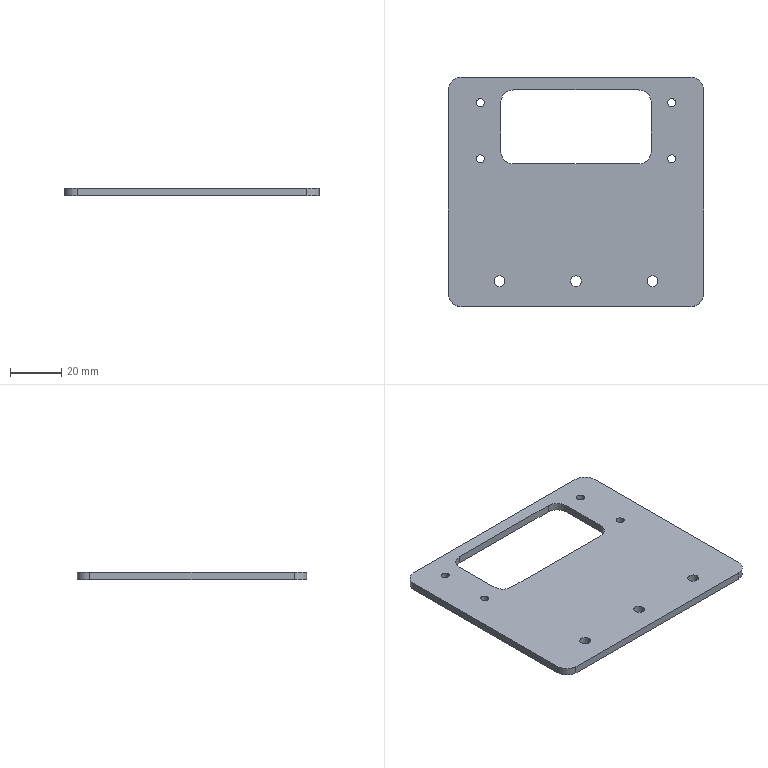Part | SolidWorks | features BaseBody 1 | 1 solid | 32 faces | box 100 x 90 x 3 mm | volume 21646 mm3 | cylinder 22 | plane 10 | commonest cylinder face diameters 3.2 x8 10 x8 4.2 x6
STEP:
#1=CARTESIAN_POINT('',(2.1,-35.,3.));
#2=VERTEX_POINT('',#1);
#3=CARTESIAN_POINT('',(-2.1,-35.,3.));
#4=VERTEX_POINT('',#3);
#5=CARTESIAN_POINT('',(0.,-35.,3.));
#6=DIRECTION('',(0.,0.,-1.));
#7=DIRECTION('',(-1.,0.,0.));
#8=AXIS2_PLACEMENT_3D('',#5,#6,#7);
#9=CIRCLE('',#8,2.1);
#10=EDGE_CURVE('',#2,#4,#9,.T.);
#11=ORIENTED_EDGE('',*,*,#10,.F.);
#12=CARTESIAN_POINT('',(2.1,-35.,0.));
#13=VERTEX_POINT('',#12);
#14=CARTESIAN_POINT('',(2.1,-35.,3.));
#15=DIRECTION('',(0.,0.,-1.));
#16=VECTOR('',#15,1000.);
#17=LINE('',#14,#16);
#18=EDGE_CURVE('',#2,#13,#17,.T.);
#19=ORIENTED_EDGE('',*,*,#18,.T.);
#20=CARTESIAN_POINT('',(-2.1,-35.,0.));
#21=VERTEX_POINT('',#20);
#22=CARTESIAN_POINT('',(0.,-35.,0.));
#23=DIRECTION('',(0.,0.,1.));
#24=DIRECTION('',(-1.,0.,0.));
#25=AXIS2_PLACEMENT_3D('',#22,#23,#24);
#26=CIRCLE('',#25,2.1);
#27=EDGE_CURVE('',#21,#13,#26,.T.);
#28=ORIENTED_EDGE('',*,*,#27,.F.);
#29=CARTESIAN_POINT('',(-2.1,-35.,3.));
#30=DIRECTION('',(0.,0.,-1.));
#31=VECTOR('',#30,1000.);
#32=LINE('',#29,#31);
#33=EDGE_CURVE('',#4,#21,#32,.T.);
#34=ORIENTED_EDGE('',*,*,#33,.F.);
#35=EDGE_LOOP('',(#11,#19,#28,#34));
#36=FACE_OUTER_BOUND('',#35,.T.);
#37=CARTESIAN_POINT('',(0.,-35.,3.));
#38=DIRECTION('',(0.,0.,-1.));
#39=DIRECTION('',(-1.,0.,0.));
#40=AXIS2_PLACEMENT_3D('',#37,#38,#39);
#41=CYLINDRICAL_SURFACE('',#40,2.1);
#42=ADVANCED_FACE('',(#36),#41,.F.);
#43=CARTESIAN_POINT('',(32.1,-35.,3.));
#44=VERTEX_POINT('',#43);
#45=CARTESIAN_POINT('',(27.9,-35.,3.));
#46=VERTEX_POINT('',#45);
#47=CARTESIAN_POINT('',(30.,-35.,3.));
#48=DIRECTION('',(0.,0.,-1.));
#49=DIRECTION('',(-1.,0.,0.));
#50=AXIS2_PLACEMENT_3D('',#47,#48,#49);
#51=CIRCLE('',#50,2.1);
#52=EDGE_CURVE('',#44,#46,#51,.T.);
#53=ORIENTED_EDGE('',*,*,#52,.F.);
#54=CARTESIAN_POINT('',(32.1,-35.,0.));
#55=VERTEX_POINT('',#54);
#56=CARTESIAN_POINT('',(32.1,-35.,3.));
#57=DIRECTION('',(0.,0.,-1.));
#58=VECTOR('',#57,1000.);
#59=LINE('',#56,#58);
#60=EDGE_CURVE('',#44,#55,#59,.T.);
#61=ORIENTED_EDGE('',*,*,#60,.T.);
#62=CARTESIAN_POINT('',(27.9,-35.,0.));
#63=VERTEX_POINT('',#62);
#64=CARTESIAN_POINT('',(30.,-35.,0.));
#65=DIRECTION('',(0.,0.,1.));
#66=DIRECTION('',(-1.,0.,0.));
#67=AXIS2_PLACEMENT_3D('',#64,#65,#66);
#68=CIRCLE('',#67,2.1);
#69=EDGE_CURVE('',#63,#55,#68,.T.);
#70=ORIENTED_EDGE('',*,*,#69,.F.);
#71=CARTESIAN_POINT('',(27.9,-35.,3.));
#72=DIRECTION('',(0.,0.,-1.));
#73=VECTOR('',#72,1000.);
#74=LINE('',#71,#73);
#75=EDGE_CURVE('',#46,#63,#74,.T.);
#76=ORIENTED_EDGE('',*,*,#75,.F.);
#77=EDGE_LOOP('',(#53,#61,#70,#76));
#78=FACE_OUTER_BOUND('',#77,.T.);
#79=CARTESIAN_POINT('',(30.,-35.,3.));
#80=DIRECTION('',(0.,0.,-1.));
#81=DIRECTION('',(-1.,0.,0.));
#82=AXIS2_PLACEMENT_3D('',#79,#80,#81);
#83=CYLINDRICAL_SURFACE('',#82,2.1);
#84=ADVANCED_FACE('',(#78),#83,.F.);
#85=CARTESIAN_POINT('',(39.1,13.,3.));
#86=VERTEX_POINT('',#85);
#87=CARTESIAN_POINT('',(35.9,13.,3.));
#88=VERTEX_POINT('',#87);
#89=CARTESIAN_POINT('',(37.5,13.,3.));
#90=DIRECTION('',(0.,0.,-1.));
#91=DIRECTION('',(-1.,0.,0.));
#92=AXIS2_PLACEMENT_3D('',#89,#90,#91);
#93=CIRCLE('',#92,1.6);
#94=EDGE_CURVE('',#86,#88,#93,.T.);
#95=ORIENTED_EDGE('',*,*,#94,.F.);
#96=CARTESIAN_POINT('',(39.1,13.,0.));
#97=VERTEX_POINT('',#96);
#98=CARTESIAN_POINT('',(39.1,13.,3.));
#99=DIRECTION('',(0.,0.,-1.));
#100=VECTOR('',#99,1000.);
#101=LINE('',#98,#100);
#102=EDGE_CURVE('',#86,#97,#101,.T.);
#103=ORIENTED_EDGE('',*,*,#102,.T.);
#104=CARTESIAN_POINT('',(35.9,13.,0.));
#105=VERTEX_POINT('',#104);
#106=CARTESIAN_POINT('',(37.5,13.,0.));
#107=DIRECTION('',(0.,0.,1.));
#108=DIRECTION('',(-1.,0.,0.));
#109=AXIS2_PLACEMENT_3D('',#106,#107,#108);
#110=CIRCLE('',#109,1.6);
#111=EDGE_CURVE('',#105,#97,#110,.T.);
#112=ORIENTED_EDGE('',*,*,#111,.F.);
#113=CARTESIAN_POINT('',(35.9,13.,3.));
#114=DIRECTION('',(0.,0.,-1.));
#115=VECTOR('',#114,1000.);
#116=LINE('',#113,#115);
#117=EDGE_CURVE('',#88,#105,#116,.T.);
#118=ORIENTED_EDGE('',*,*,#117,.F.);
#119=EDGE_LOOP('',(#95,#103,#112,#118));
#120=FACE_OUTER_BOUND('',#119,.T.);
#121=CARTESIAN_POINT('',(37.5,13.,3.));
#122=DIRECTION('',(0.,0.,-1.));
#123=DIRECTION('',(-1.,0.,0.));
#124=AXIS2_PLACEMENT_3D('',#121,#122,#123);
#125=CYLINDRICAL_SURFACE('',#124,1.6);
#126=ADVANCED_FACE('',(#120),#125,.F.);
#127=CARTESIAN_POINT('',(-35.9,13.,3.));
#128=VERTEX_POINT('',#127);
#129=CARTESIAN_POINT('',(-39.1,13.,3.));
#130=VERTEX_POINT('',#129);
#131=CARTESIAN_POINT('',(-37.5,13.,3.));
#132=DIRECTION('',(0.,0.,-1.));
#133=DIRECTION('',(-1.,0.,0.));
#134=AXIS2_PLACEMENT_3D('',#131,#132,#133);
#135=CIRCLE('',#134,1.6);
#136=EDGE_CURVE('',#128,#130,#135,.T.);
#137=ORIENTED_EDGE('',*,*,#136,.F.);
#138=CARTESIAN_POINT('',(-35.9,13.,0.));
#139=VERTEX_POINT('',#138);
#140=CARTESIAN_POINT('',(-35.9,13.,3.));
#141=DIRECTION('',(0.,0.,-1.));
#142=VECTOR('',#141,1000.);
#143=LINE('',#140,#142);
#144=EDGE_CURVE('',#128,#139,#143,.T.);
#145=ORIENTED_EDGE('',*,*,#144,.T.);
#146=CARTESIAN_POINT('',(-39.1,13.,0.));
#147=VERTEX_POINT('',#146);
#148=CARTESIAN_POINT('',(-37.5,13.,0.));
#149=DIRECTION('',(0.,0.,1.));
#150=DIRECTION('',(-1.,0.,0.));
#151=AXIS2_PLACEMENT_3D('',#148,#149,#150);
#152=CIRCLE('',#151,1.6);
#153=EDGE_CURVE('',#147,#139,#152,.T.);
#154=ORIENTED_EDGE('',*,*,#153,.F.);
#155=CARTESIAN_POINT('',(-39.1,13.,3.));
#156=DIRECTION('',(0.,0.,-1.));
#157=VECTOR('',#156,1000.);
#158=LINE('',#155,#157);
#159=EDGE_CURVE('',#130,#147,#158,.T.);
#160=ORIENTED_EDGE('',*,*,#159,.F.);
#161=EDGE_LOOP('',(#137,#145,#154,#160));
#162=FACE_OUTER_BOUND('',#161,.T.);
#163=CARTESIAN_POINT('',(-37.5,13.,3.));
#164=DIRECTION('',(0.,0.,-1.));
#165=DIRECTION('',(-1.,0.,0.));
#166=AXIS2_PLACEMENT_3D('',#163,#164,#165);
#167=CYLINDRICAL_SURFACE('',#166,1.6);
#168=ADVANCED_FACE('',(#162),#167,.F.);
#169=CARTESIAN_POINT('',(-35.9,35.,3.));
#170=VERTEX_POINT('',#169);
#171=CARTESIAN_POINT('',(-39.1,35.,3.));
#172=VERTEX_POINT('',#171);
#173=CARTESIAN_POINT('',(-37.5,35.,3.));
#174=DIRECTION('',(0.,0.,-1.));
#175=DIRECTION('',(-1.,0.,0.));
#176=AXIS2_PLACEMENT_3D('',#173,#174,#175);
#177=CIRCLE('',#176,1.6);
#178=EDGE_CURVE('',#170,#172,#177,.T.);
#179=ORIENTED_EDGE('',*,*,#178,.F.);
#180=CARTESIAN_POINT('',(-35.9,35.,0.));
#181=VERTEX_POINT('',#180);
#182=CARTESIAN_POINT('',(-35.9,35.,3.));
#183=DIRECTION('',(0.,0.,-1.));
#184=VECTOR('',#183,1000.);
#185=LINE('',#182,#184);
#186=EDGE_CURVE('',#170,#181,#185,.T.);
#187=ORIENTED_EDGE('',*,*,#186,.T.);
#188=CARTESIAN_POINT('',(-39.1,35.,0.));
#189=VERTEX_POINT('',#188);
#190=CARTESIAN_POINT('',(-37.5,35.,0.));
#191=DIRECTION('',(0.,0.,1.));
#192=DIRECTION('',(-1.,0.,0.));
#193=AXIS2_PLACEMENT_3D('',#190,#191,#192);
#194=CIRCLE('',#193,1.6);
#195=EDGE_CURVE('',#189,#181,#194,.T.);
#196=ORIENTED_EDGE('',*,*,#195,.F.);
#197=CARTESIAN_POINT('',(-39.1,35.,3.));
#198=DIRECTION('',(0.,0.,-1.));
#199=VECTOR('',#198,1000.);
#200=LINE('',#197,#199);
#201=EDGE_CURVE('',#172,#189,#200,.T.);
#202=ORIENTED_EDGE('',*,*,#201,.F.);
#203=EDGE_LOOP('',(#179,#187,#196,#202));
#204=FACE_OUTER_BOUND('',#203,.T.);
#205=CARTESIAN_POINT('',(-37.5,35.,3.));
#206=DIRECTION('',(0.,0.,-1.));
#207=DIRECTION('',(-1.,0.,0.));
#208=AXIS2_PLACEMENT_3D('',#205,#206,#207);
#209=CYLINDRICAL_SURFACE('',#208,1.6);
#210=ADVANCED_FACE('',(#204),#209,.F.);
#211=CARTESIAN_POINT('',(39.1,35.,3.));
#212=VERTEX_POINT('',#211);
#213=CARTESIAN_POINT('',(35.9,35.,3.));
#214=VERTEX_POINT('',#213);
#215=CARTESIAN_POINT('',(37.5,35.,3.));
#216=DIRECTION('',(0.,0.,-1.));
#217=DIRECTION('',(-1.,0.,0.));
#218=AXIS2_PLACEMENT_3D('',#215,#216,#217);
#219=CIRCLE('',#218,1.6);
#220=EDGE_CURVE('',#212,#214,#219,.T.);
#221=ORIENTED_EDGE('',*,*,#220,.F.);
#222=CARTESIAN_POINT('',(39.1,35.,0.));
#223=VERTEX_POINT('',#222);
#224=CARTESIAN_POINT('',(39.1,35.,3.));
#225=DIRECTION('',(0.,0.,-1.));
#226=VECTOR('',#225,1000.);
#227=LINE('',#224,#226);
#228=EDGE_CURVE('',#212,#223,#227,.T.);
#229=ORIENTED_EDGE('',*,*,#228,.T.);
#230=CARTESIAN_POINT('',(35.9,35.,0.));
#231=VERTEX_POINT('',#230);
#232=CARTESIAN_POINT('',(37.5,35.,0.));
#233=DIRECTION('',(0.,0.,1.));
#234=DIRECTION('',(-1.,0.,0.));
#235=AXIS2_PLACEMENT_3D('',#232,#233,#234);
#236=CIRCLE('',#235,1.6);
#237=EDGE_CURVE('',#231,#223,#236,.T.);
#238=ORIENTED_EDGE('',*,*,#237,.F.);
#239=CARTESIAN_POINT('',(35.9,35.,3.));
#240=DIRECTION('',(0.,0.,-1.));
#241=VECTOR('',#240,1000.);
#242=LINE('',#239,#241);
#243=EDGE_CURVE('',#214,#231,#242,.T.);
#244=ORIENTED_EDGE('',*,*,#243,.F.);
#245=EDGE_LOOP('',(#221,#229,#238,#244));
#246=FACE_OUTER_BOUND('',#245,.T.);
#247=CARTESIAN_POINT('',(37.5,35.,3.));
#248=DIRECTION('',(0.,0.,-1.));
#249=DIRECTION('',(-1.,0.,0.));
#250=AXIS2_PLACEMENT_3D('',#247,#248,#249);
#251=CYLINDRICAL_SURFACE('',#250,1.6);
#252=ADVANCED_FACE('',(#246),#251,.F.);
#253=CARTESIAN_POINT('',(-27.9,-35.,3.));
#254=VERTEX_POINT('',#253);
#255=CARTESIAN_POINT('',(-32.1,-35.,3.));
#256=VERTEX_POINT('',#255);
#257=CARTESIAN_POINT('',(-30.,-35.,3.));
#258=DIRECTION('',(0.,0.,-1.));
#259=DIRECTION('',(-1.,0.,0.));
#260=AXIS2_PLACEMENT_3D('',#257,#258,#259);
#261=CIRCLE('',#260,2.1);
#262=EDGE_CURVE('',#254,#256,#261,.T.);
#263=ORIENTED_EDGE('',*,*,#262,.F.);
#264=CARTESIAN_POINT('',(-27.9,-35.,0.));
#265=VERTEX_POINT('',#264);
#266=CARTESIAN_POINT('',(-27.9,-35.,3.));
#267=DIRECTION('',(0.,0.,-1.));
#268=VECTOR('',#267,1000.);
#269=LINE('',#266,#268);
#270=EDGE_CURVE('',#254,#265,#269,.T.);
#271=ORIENTED_EDGE('',*,*,#270,.T.);
#272=CARTESIAN_POINT('',(-32.1,-35.,0.));
#273=VERTEX_POINT('',#272);
#274=CARTESIAN_POINT('',(-30.,-35.,0.));
#275=DIRECTION('',(0.,0.,1.));
#276=DIRECTION('',(-1.,0.,0.));
#277=AXIS2_PLACEMENT_3D('',#274,#275,#276);
#278=CIRCLE('',#277,2.1);
#279=EDGE_CURVE('',#273,#265,#278,.T.);
#280=ORIENTED_EDGE('',*,*,#279,.F.);
#281=CARTESIAN_POINT('',(-32.1,-35.,3.));
#282=DIRECTION('',(0.,0.,-1.));
#283=VECTOR('',#282,1000.);
#284=LINE('',#281,#283);
#285=EDGE_CURVE('',#256,#273,#284,.T.);
#286=ORIENTED_EDGE('',*,*,#285,.F.);
#287=EDGE_LOOP('',(#263,#271,#280,#286));
#288=FACE_OUTER_BOUND('',#287,.T.);
#289=CARTESIAN_POINT('',(-30.,-35.,3.));
#290=DIRECTION('',(0.,0.,-1.));
#291=DIRECTION('',(-1.,0.,0.));
#292=AXIS2_PLACEMENT_3D('',#289,#290,#291);
#293=CYLINDRICAL_SURFACE('',#292,2.1);
#294=ADVANCED_FACE('',(#288),#293,.F.);
#295=ORIENTED_EDGE('',*,*,#27,.T.);
#296=CARTESIAN_POINT('',(0.,-35.,0.));
#297=DIRECTION('',(0.,0.,1.));
#298=DIRECTION('',(-1.,0.,0.));
#299=AXIS2_PLACEMENT_3D('',#296,#297,#298);
#300=CIRCLE('',#299,2.1);
#301=EDGE_CURVE('',#13,#21,#300,.T.);
#302=ORIENTED_EDGE('',*,*,#301,.T.);
#303=EDGE_LOOP('',(#295,#302));
#304=FACE_BOUND('',#303,.T.);
#305=ORIENTED_EDGE('',*,*,#69,.T.);
#306=CARTESIAN_POINT('',(30.,-35.,0.));
#307=DIRECTION('',(0.,0.,1.));
#308=DIRECTION('',(-1.,0.,0.));
#309=AXIS2_PLACEMENT_3D('',#306,#307,#308);
#310=CIRCLE('',#309,2.1);
#311=EDGE_CURVE('',#55,#63,#310,.T.);
#312=ORIENTED_EDGE('',*,*,#311,.T.);
#313=EDGE_LOOP('',(#305,#312));
#314=FACE_BOUND('',#313,.T.);
#315=ORIENTED_EDGE('',*,*,#111,.T.);
#316=CARTESIAN_POINT('',(37.5,13.,0.));
#317=DIRECTION('',(0.,0.,1.));
#318=DIRECTION('',(-1.,0.,0.));
#319=AXIS2_PLACEMENT_3D('',#316,#317,#318);
#320=CIRCLE('',#319,1.6);
#321=EDGE_CURVE('',#97,#105,#320,.T.);
#322=ORIENTED_EDGE('',*,*,#321,.T.);
#323=EDGE_LOOP('',(#315,#322));
#324=FACE_BOUND('',#323,.T.);
#325=ORIENTED_EDGE('',*,*,#153,.T.);
#326=CARTESIAN_POINT('',(-37.5,13.,0.));
#327=DIRECTION('',(0.,0.,1.));
#328=DIRECTION('',(-1.,0.,0.));
#329=AXIS2_PLACEMENT_3D('',#326,#327,#328);
#330=CIRCLE('',#329,1.6);
#331=EDGE_CURVE('',#139,#147,#330,.T.);
#332=ORIENTED_EDGE('',*,*,#331,.T.);
#333=EDGE_LOOP('',(#325,#332));
#334=FACE_BOUND('',#333,.T.);
#335=CARTESIAN_POINT('',(-45.,45.,0.));
#336=VERTEX_POINT('',#335);
#337=CARTESIAN_POINT('',(45.,45.,0.));
#338=VERTEX_POINT('',#337);
#339=CARTESIAN_POINT('',(0.,45.,0.));
#340=DIRECTION('',(1.,0.,0.));
#341=VECTOR('',#340,1000.);
#342=LINE('',#339,#341);
#343=EDGE_CURVE('',#336,#338,#342,.T.);
#344=ORIENTED_EDGE('',*,*,#343,.T.);
#345=CARTESIAN_POINT('',(50.,40.,0.));
#346=VERTEX_POINT('',#345);
#347=CARTESIAN_POINT('',(45.,40.,0.));
#348=DIRECTION('',(0.,0.,-1.));
#349=DIRECTION('',(-1.,0.,0.));
#350=AXIS2_PLACEMENT_3D('',#347,#348,#349);
#351=CIRCLE('',#350,5.);
#352=EDGE_CURVE('',#338,#346,#351,.T.);
#353=ORIENTED_EDGE('',*,*,#352,.T.);
#354=CARTESIAN_POINT('',(50.,-40.,0.));
#355=VERTEX_POINT('',#354);
#356=CARTESIAN_POINT('',(50.,0.,0.));
#357=DIRECTION('',(0.,-1.,0.));
#358=VECTOR('',#357,1000.);
#359=LINE('',#356,#358);
#360=EDGE_CURVE('',#346,#355,#359,.T.);
#361=ORIENTED_EDGE('',*,*,#360,.T.);
#362=CARTESIAN_POINT('',(45.,-45.,0.));
#363=VERTEX_POINT('',#362);
#364=CARTESIAN_POINT('',(45.,-40.,0.));
#365=DIRECTION('',(0.,0.,-1.));
#366=DIRECTION('',(-1.,0.,0.));
#367=AXIS2_PLACEMENT_3D('',#364,#365,#366);
#368=CIRCLE('',#367,5.);
#369=EDGE_CURVE('',#355,#363,#368,.T.);
#370=ORIENTED_EDGE('',*,*,#369,.T.);
#371=CARTESIAN_POINT('',(-45.,-45.,0.));
#372=VERTEX_POINT('',#371);
#373=CARTESIAN_POINT('',(0.,-45.,0.));
#374=DIRECTION('',(-1.,0.,0.));
#375=VECTOR('',#374,1000.);
#376=LINE('',#373,#375);
#377=EDGE_CURVE('',#363,#372,#376,.T.);
#378=ORIENTED_EDGE('',*,*,#377,.T.);
#379=CARTESIAN_POINT('',(-50.,-40.,0.));
#380=VERTEX_POINT('',#379);
#381=CARTESIAN_POINT('',(-45.,-40.,0.));
#382=DIRECTION('',(0.,0.,-1.));
#383=DIRECTION('',(-1.,0.,0.));
#384=AXIS2_PLACEMENT_3D('',#381,#382,#383);
#385=CIRCLE('',#384,5.);
#386=EDGE_CURVE('',#372,#380,#385,.T.);
#387=ORIENTED_EDGE('',*,*,#386,.T.);
#388=CARTESIAN_POINT('',(-50.,40.,0.));
#389=VERTEX_POINT('',#388);
#390=CARTESIAN_POINT('',(-50.,0.,0.));
#391=DIRECTION('',(0.,1.,0.));
#392=VECTOR('',#391,1000.);
#393=LINE('',#390,#392);
#394=EDGE_CURVE('',#380,#389,#393,.T.);
#395=ORIENTED_EDGE('',*,*,#394,.T.);
#396=CARTESIAN_POINT('',(-45.,40.,0.));
#397=DIRECTION('',(0.,0.,-1.));
#398=DIRECTION('',(-1.,0.,0.));
#399=AXIS2_PLACEMENT_3D('',#396,#397,#398);
#400=CIRCLE('',#399,5.);
#401=EDGE_CURVE('',#389,#336,#400,.T.);
#402=ORIENTED_EDGE('',*,*,#401,.T.);
#403=EDGE_LOOP('',(#344,#353,#361,#370,#378,#387,#395,#402));
#404=FACE_OUTER_BOUND('',#403,.T.);
#405=ORIENTED_EDGE('',*,*,#195,.T.);
#406=CARTESIAN_POINT('',(-37.5,35.,0.));
#407=DIRECTION('',(0.,0.,1.));
#408=DIRECTION('',(-1.,0.,0.));
#409=AXIS2_PLACEMENT_3D('',#406,#407,#408);
#410=CIRCLE('',#409,1.6);
#411=EDGE_CURVE('',#181,#189,#410,.T.);
#412=ORIENTED_EDGE('',*,*,#411,.T.);
#413=EDGE_LOOP('',(#405,#412));
#414=FACE_BOUND('',#413,.T.);
#415=ORIENTED_EDGE('',*,*,#237,.T.);
#416=CARTESIAN_POINT('',(37.5,35.,0.));
#417=DIRECTION('',(0.,0.,1.));
#418=DIRECTION('',(-1.,0.,0.));
#419=AXIS2_PLACEMENT_3D('',#416,#417,#418);
#420=CIRCLE('',#419,1.6);
#421=EDGE_CURVE('',#223,#231,#420,.T.);
#422=ORIENTED_EDGE('',*,*,#421,.T.);
#423=EDGE_LOOP('',(#415,#422));
#424=FACE_BOUND('',#423,.T.);
#425=ORIENTED_EDGE('',*,*,#279,.T.);
#426=CARTESIAN_POINT('',(-30.,-35.,0.));
#427=DIRECTION('',(0.,0.,1.));
#428=DIRECTION('',(-1.,0.,0.));
#429=AXIS2_PLACEMENT_3D('',#426,#427,#428);
#430=CIRCLE('',#429,2.1);
#431=EDGE_CURVE('',#265,#273,#430,.T.);
#432=ORIENTED_EDGE('',*,*,#431,.T.);
#433=EDGE_LOOP('',(#425,#432));
#434=FACE_BOUND('',#433,.T.);
#435=CARTESIAN_POINT('',(-24.5,11.,0.));
#436=VERTEX_POINT('',#435);
#437=CARTESIAN_POINT('',(24.5,11.,0.));
#438=VERTEX_POINT('',#437);
#439=CARTESIAN_POINT('',(0.,11.,0.));
#440=DIRECTION('',(1.,0.,0.));
#441=VECTOR('',#440,1000.);
#442=LINE('',#439,#441);
#443=EDGE_CURVE('',#436,#438,#442,.T.);
#444=ORIENTED_EDGE('',*,*,#443,.T.);
#445=CARTESIAN_POINT('',(29.5,16.,0.));
#446=VERTEX_POINT('',#445);
#447=CARTESIAN_POINT('',(24.5,16.,0.));
#448=DIRECTION('',(0.,0.,1.));
#449=DIRECTION('',(-1.,0.,0.));
#450=AXIS2_PLACEMENT_3D('',#447,#448,#449);
#451=CIRCLE('',#450,5.);
#452=EDGE_CURVE('',#438,#446,#451,.T.);
#453=ORIENTED_EDGE('',*,*,#452,.T.);
#454=CARTESIAN_POINT('',(29.5,35.,0.));
#455=VERTEX_POINT('',#454);
#456=CARTESIAN_POINT('',(29.5,0.,0.));
#457=DIRECTION('',(0.,1.,0.));
#458=VECTOR('',#457,1000.);
#459=LINE('',#456,#458);
#460=EDGE_CURVE('',#446,#455,#459,.T.);
#461=ORIENTED_EDGE('',*,*,#460,.T.);
#462=CARTESIAN_POINT('',(24.5,40.,0.));
#463=VERTEX_POINT('',#462);
#464=CARTESIAN_POINT('',(24.5,35.,0.));
#465=DIRECTION('',(0.,0.,1.));
#466=DIRECTION('',(-1.,0.,0.));
#467=AXIS2_PLACEMENT_3D('',#464,#465,#466);
#468=CIRCLE('',#467,5.);
#469=EDGE_CURVE('',#455,#463,#468,.T.);
#470=ORIENTED_EDGE('',*,*,#469,.T.);
#471=CARTESIAN_POINT('',(-24.5,40.,0.));
#472=VERTEX_POINT('',#471);
#473=CARTESIAN_POINT('',(0.,40.,0.));
#474=DIRECTION('',(-1.,0.,0.));
#475=VECTOR('',#474,1000.);
#476=LINE('',#473,#475);
#477=EDGE_CURVE('',#463,#472,#476,.T.);
#478=ORIENTED_EDGE('',*,*,#477,.T.);
#479=CARTESIAN_POINT('',(-29.5,35.,0.));
#480=VERTEX_POINT('',#479);
#481=CARTESIAN_POINT('',(-24.5,35.,0.));
#482=DIRECTION('',(0.,0.,1.));
#483=DIRECTION('',(-1.,0.,0.));
#484=AXIS2_PLACEMENT_3D('',#481,#482,#483);
#485=CIRCLE('',#484,5.);
#486=EDGE_CURVE('',#472,#480,#485,.T.);
#487=ORIENTED_EDGE('',*,*,#486,.T.);
#488=CARTESIAN_POINT('',(-29.5,16.,0.));
#489=VERTEX_POINT('',#488);
#490=CARTESIAN_POINT('',(-29.5,0.,0.));
#491=DIRECTION('',(0.,-1.,0.));
#492=VECTOR('',#491,1000.);
#493=LINE('',#490,#492);
#494=EDGE_CURVE('',#480,#489,#493,.T.);
#495=ORIENTED_EDGE('',*,*,#494,.T.);
#496=CARTESIAN_POINT('',(-24.5,16.,0.));
#497=DIRECTION('',(0.,0.,1.));
#498=DIRECTION('',(-1.,0.,0.));
#499=AXIS2_PLACEMENT_3D('',#496,#497,#498);
#500=CIRCLE('',#499,5.);
#501=EDGE_CURVE('',#489,#436,#500,.T.);
#502=ORIENTED_EDGE('',*,*,#501,.T.);
#503=EDGE_LOOP('',(#444,#453,#461,#470,#478,#487,#495,#502));
#504=FACE_BOUND('',#503,.T.);
#505=CARTESIAN_POINT('',(0.,0.,0.));
#506=DIRECTION('',(0.,0.,-1.));
#507=DIRECTION('',(-1.,0.,0.));
#508=AXIS2_PLACEMENT_3D('',#505,#506,#507);
#509=PLANE('',#508);
#510=ADVANCED_FACE('',(#304,#314,#324,#334,#404,#414,#424,#434,#504),#509,.T.);
#511=ORIENTED_EDGE('',*,*,#18,.F.);
#512=CARTESIAN_POINT('',(0.,-35.,3.));
#513=DIRECTION('',(0.,0.,-1.));
#514=DIRECTION('',(-1.,0.,0.));
#515=AXIS2_PLACEMENT_3D('',#512,#513,#514);
#516=CIRCLE('',#515,2.1);
#517=EDGE_CURVE('',#4,#2,#516,.T.);
#518=ORIENTED_EDGE('',*,*,#517,.F.);
#519=ORIENTED_EDGE('',*,*,#33,.T.);
#520=ORIENTED_EDGE('',*,*,#301,.F.);
#521=EDGE_LOOP('',(#511,#518,#519,#520));
#522=FACE_OUTER_BOUND('',#521,.T.);
#523=CARTESIAN_POINT('',(0.,-35.,3.));
#524=DIRECTION('',(0.,0.,-1.));
#525=DIRECTION('',(-1.,0.,0.));
#526=AXIS2_PLACEMENT_3D('',#523,#524,#525);
#527=CYLINDRICAL_SURFACE('',#526,2.1);
#528=ADVANCED_FACE('',(#522),#527,.F.);
#529=ORIENTED_EDGE('',*,*,#60,.F.);
#530=CARTESIAN_POINT('',(30.,-35.,3.));
#531=DIRECTION('',(0.,0.,-1.));
#532=DIRECTION('',(-1.,0.,0.));
#533=AXIS2_PLACEMENT_3D('',#530,#531,#532);
#534=CIRCLE('',#533,2.1);
#535=EDGE_CURVE('',#46,#44,#534,.T.);
#536=ORIENTED_EDGE('',*,*,#535,.F.);
#537=ORIENTED_EDGE('',*,*,#75,.T.);
#538=ORIENTED_EDGE('',*,*,#311,.F.);
#539=EDGE_LOOP('',(#529,#536,#537,#538));
#540=FACE_OUTER_BOUND('',#539,.T.);
#541=CARTESIAN_POINT('',(30.,-35.,3.));
#542=DIRECTION('',(0.,0.,-1.));
#543=DIRECTION('',(-1.,0.,0.));
#544=AXIS2_PLACEMENT_3D('',#541,#542,#543);
#545=CYLINDRICAL_SURFACE('',#544,2.1);
#546=ADVANCED_FACE('',(#540),#545,.F.);
#547=ORIENTED_EDGE('',*,*,#102,.F.);
#548=CARTESIAN_POINT('',(37.5,13.,3.));
#549=DIRECTION('',(0.,0.,-1.));
#550=DIRECTION('',(-1.,0.,0.));
#551=AXIS2_PLACEMENT_3D('',#548,#549,#550);
#552=CIRCLE('',#551,1.6);
#553=EDGE_CURVE('',#88,#86,#552,.T.);
#554=ORIENTED_EDGE('',*,*,#553,.F.);
#555=ORIENTED_EDGE('',*,*,#117,.T.);
#556=ORIENTED_EDGE('',*,*,#321,.F.);
#557=EDGE_LOOP('',(#547,#554,#555,#556));
#558=FACE_OUTER_BOUND('',#557,.T.);
#559=CARTESIAN_POINT('',(37.5,13.,3.));
#560=DIRECTION('',(0.,0.,-1.));
#561=DIRECTION('',(-1.,0.,0.));
#562=AXIS2_PLACEMENT_3D('',#559,#560,#561);
#563=CYLINDRICAL_SURFACE('',#562,1.6);
#564=ADVANCED_FACE('',(#558),#563,.F.);
#565=ORIENTED_EDGE('',*,*,#144,.F.);
#566=CARTESIAN_POINT('',(-37.5,13.,3.));
#567=DIRECTION('',(0.,0.,-1.));
#568=DIRECTION('',(-1.,0.,0.));
#569=AXIS2_PLACEMENT_3D('',#566,#567,#568);
#570=CIRCLE('',#569,1.6);
#571=EDGE_CURVE('',#130,#128,#570,.T.);
#572=ORIENTED_EDGE('',*,*,#571,.F.);
#573=ORIENTED_EDGE('',*,*,#159,.T.);
#574=ORIENTED_EDGE('',*,*,#331,.F.);
#575=EDGE_LOOP('',(#565,#572,#573,#574));
#576=FACE_OUTER_BOUND('',#575,.T.);
#577=CARTESIAN_POINT('',(-37.5,13.,3.));
#578=DIRECTION('',(0.,0.,-1.));
#579=DIRECTION('',(-1.,0.,0.));
#580=AXIS2_PLACEMENT_3D('',#577,#578,#579);
#581=CYLINDRICAL_SURFACE('',#580,1.6);
#582=ADVANCED_FACE('',(#576),#581,.F.);
#583=ORIENTED_EDGE('',*,*,#352,.F.);
#584=CARTESIAN_POINT('',(45.,45.,3.));
#585=VERTEX_POINT('',#584);
#586=CARTESIAN_POINT('',(45.,45.,3.));
#587=DIRECTION('',(0.,0.,1.));
#588=VECTOR('',#587,1000.);
#589=LINE('',#586,#588);
#590=EDGE_CURVE('',#338,#585,#589,.T.);
#591=ORIENTED_EDGE('',*,*,#590,.T.);
#592=CARTESIAN_POINT('',(50.,40.,3.));
#593=VERTEX_POINT('',#592);
#594=CARTESIAN_POINT('',(45.,40.,3.));
#595=DIRECTION('',(0.,0.,-1.));
#596=DIRECTION('',(-1.,0.,0.));
#597=AXIS2_PLACEMENT_3D('',#594,#595,#596);
#598=CIRCLE('',#597,5.);
#599=EDGE_CURVE('',#585,#593,#598,.T.);
#600=ORIENTED_EDGE('',*,*,#599,.T.);
#601=CARTESIAN_POINT('',(50.,40.,3.));
#602=DIRECTION('',(0.,0.,-1.));
#603=VECTOR('',#602,1000.);
#604=LINE('',#601,#603);
#605=EDGE_CURVE('',#593,#346,#604,.T.);
#606=ORIENTED_EDGE('',*,*,#605,.T.);
#607=EDGE_LOOP('',(#583,#591,#600,#606));
#608=FACE_OUTER_BOUND('',#607,.T.);
#609=CARTESIAN_POINT('',(45.,40.,3.));
#610=DIRECTION('',(0.,0.,-1.));
#611=DIRECTION('',(-1.,0.,0.));
#612=AXIS2_PLACEMENT_3D('',#609,#610,#611);
#613=CYLINDRICAL_SURFACE('',#612,5.);
#614=ADVANCED_FACE('',(#608),#613,.T.);
#615=CARTESIAN_POINT('',(-45.,45.,3.));
#616=VERTEX_POINT('',#615);
#617=CARTESIAN_POINT('',(-45.,45.,3.));
#618=DIRECTION('',(0.,0.,-1.));
#619=VECTOR('',#618,1000.);
#620=LINE('',#617,#619);
#621=EDGE_CURVE('',#616,#336,#620,.T.);
#622=ORIENTED_EDGE('',*,*,#621,.F.);
#623=CARTESIAN_POINT('',(-50.,45.,3.));
#624=DIRECTION('',(-1.,0.,0.));
#625=VECTOR('',#624,1000.);
#626=LINE('',#623,#625);
#627=EDGE_CURVE('',#585,#616,#626,.T.);
#628=ORIENTED_EDGE('',*,*,#627,.F.);
#629=ORIENTED_EDGE('',*,*,#590,.F.);
#630=ORIENTED_EDGE('',*,*,#343,.F.);
#631=EDGE_LOOP('',(#622,#628,#629,#630));
#632=FACE_OUTER_BOUND('',#631,.T.);
#633=CARTESIAN_POINT('',(-50.,45.,3.));
#634=DIRECTION('',(0.,-1.,0.));
#635=DIRECTION('',(0.,0.,-1.));
#636=AXIS2_PLACEMENT_3D('',#633,#634,#635);
#637=PLANE('',#636);
#638=ADVANCED_FACE('',(#632),#637,.F.);
#639=ORIENTED_EDGE('',*,*,#401,.F.);
#640=CARTESIAN_POINT('',(-50.,40.,3.));
#641=VERTEX_POINT('',#640);
#642=CARTESIAN_POINT('',(-50.,40.,3.));
#643=DIRECTION('',(0.,0.,1.));
#644=VECTOR('',#643,1000.);
#645=LINE('',#642,#644);
#646=EDGE_CURVE('',#389,#641,#645,.T.);
#647=ORIENTED_EDGE('',*,*,#646,.T.);
#648=CARTESIAN_POINT('',(-45.,40.,3.));
#649=DIRECTION('',(0.,0.,-1.));
#650=DIRECTION('',(-1.,0.,0.));
#651=AXIS2_PLACEMENT_3D('',#648,#649,#650);
#652=CIRCLE('',#651,5.);
#653=EDGE_CURVE('',#641,#616,#652,.T.);
#654=ORIENTED_EDGE('',*,*,#653,.T.);
#655=ORIENTED_EDGE('',*,*,#621,.T.);
#656=EDGE_LOOP('',(#639,#647,#654,#655));
#657=FACE_OUTER_BOUND('',#656,.T.);
#658=CARTESIAN_POINT('',(-45.,40.,3.));
#659=DIRECTION('',(0.,0.,-1.));
#660=DIRECTION('',(-1.,0.,0.));
#661=AXIS2_PLACEMENT_3D('',#658,#659,#660);
#662=CYLINDRICAL_SURFACE('',#661,5.);
#663=ADVANCED_FACE('',(#657),#662,.T.);
#664=CARTESIAN_POINT('',(-50.,-40.,3.));
#665=VERTEX_POINT('',#664);
#666=CARTESIAN_POINT('',(-50.,-40.,3.));
#667=DIRECTION('',(0.,0.,-1.));
#668=VECTOR('',#667,1000.);
#669=LINE('',#666,#668);
#670=EDGE_CURVE('',#665,#380,#669,.T.);
#671=ORIENTED_EDGE('',*,*,#670,.F.);
#672=CARTESIAN_POINT('',(-50.,-45.,3.));
#673=DIRECTION('',(0.,-1.,0.));
#674=VECTOR('',#673,1000.);
#675=LINE('',#672,#674);
#676=EDGE_CURVE('',#641,#665,#675,.T.);
#677=ORIENTED_EDGE('',*,*,#676,.F.);
#678=ORIENTED_EDGE('',*,*,#646,.F.);
#679=ORIENTED_EDGE('',*,*,#394,.F.);
#680=EDGE_LOOP('',(#671,#677,#678,#679));
#681=FACE_OUTER_BOUND('',#680,.T.);
#682=CARTESIAN_POINT('',(-50.,-45.,3.));
#683=DIRECTION('',(1.,0.,0.));
#684=DIRECTION('',(0.,0.,-1.));
#685=AXIS2_PLACEMENT_3D('',#682,#683,#684);
#686=PLANE('',#685);
#687=ADVANCED_FACE('',(#681),#686,.F.);
#688=ORIENTED_EDGE('',*,*,#386,.F.);
#689=CARTESIAN_POINT('',(-45.,-45.,3.));
#690=VERTEX_POINT('',#689);
#691=CARTESIAN_POINT('',(-45.,-45.,3.));
#692=DIRECTION('',(0.,0.,1.));
#693=VECTOR('',#692,1000.);
#694=LINE('',#691,#693);
#695=EDGE_CURVE('',#372,#690,#694,.T.);
#696=ORIENTED_EDGE('',*,*,#695,.T.);
#697=CARTESIAN_POINT('',(-45.,-40.,3.));
#698=DIRECTION('',(0.,0.,-1.));
#699=DIRECTION('',(-1.,0.,0.));
#700=AXIS2_PLACEMENT_3D('',#697,#698,#699);
#701=CIRCLE('',#700,5.);
#702=EDGE_CURVE('',#690,#665,#701,.T.);
#703=ORIENTED_EDGE('',*,*,#702,.T.);
#704=ORIENTED_EDGE('',*,*,#670,.T.);
#705=EDGE_LOOP('',(#688,#696,#703,#704));
#706=FACE_OUTER_BOUND('',#705,.T.);
#707=CARTESIAN_POINT('',(-45.,-40.,3.));
#708=DIRECTION('',(0.,0.,-1.));
#709=DIRECTION('',(-1.,0.,0.));
#710=AXIS2_PLACEMENT_3D('',#707,#708,#709);
#711=CYLINDRICAL_SURFACE('',#710,5.);
#712=ADVANCED_FACE('',(#706),#711,.T.);
#713=CARTESIAN_POINT('',(45.,-45.,3.));
#714=VERTEX_POINT('',#713);
#715=CARTESIAN_POINT('',(45.,-45.,3.));
#716=DIRECTION('',(0.,0.,-1.));
#717=VECTOR('',#716,1000.);
#718=LINE('',#715,#717);
#719=EDGE_CURVE('',#714,#363,#718,.T.);
#720=ORIENTED_EDGE('',*,*,#719,.F.);
#721=CARTESIAN_POINT('',(-50.,-45.,3.));
#722=DIRECTION('',(1.,0.,0.));
#723=VECTOR('',#722,1000.);
#724=LINE('',#721,#723);
#725=EDGE_CURVE('',#690,#714,#724,.T.);
#726=ORIENTED_EDGE('',*,*,#725,.F.);
#727=ORIENTED_EDGE('',*,*,#695,.F.);
#728=ORIENTED_EDGE('',*,*,#377,.F.);
#729=EDGE_LOOP('',(#720,#726,#727,#728));
#730=FACE_OUTER_BOUND('',#729,.T.);
#731=CARTESIAN_POINT('',(-50.,-45.,3.));
#732=DIRECTION('',(0.,1.,0.));
#733=DIRECTION('',(0.,0.,1.));
#734=AXIS2_PLACEMENT_3D('',#731,#732,#733);
#735=PLANE('',#734);
#736=ADVANCED_FACE('',(#730),#735,.F.);
#737=ORIENTED_EDGE('',*,*,#369,.F.);
#738=CARTESIAN_POINT('',(50.,-40.,3.));
#739=VERTEX_POINT('',#738);
#740=CARTESIAN_POINT('',(50.,-40.,3.));
#741=DIRECTION('',(0.,0.,1.));
#742=VECTOR('',#741,1000.);
#743=LINE('',#740,#742);
#744=EDGE_CURVE('',#355,#739,#743,.T.);
#745=ORIENTED_EDGE('',*,*,#744,.T.);
#746=CARTESIAN_POINT('',(45.,-40.,3.));
#747=DIRECTION('',(0.,0.,-1.));
#748=DIRECTION('',(-1.,0.,0.));
#749=AXIS2_PLACEMENT_3D('',#746,#747,#748);
#750=CIRCLE('',#749,5.);
#751=EDGE_CURVE('',#739,#714,#750,.T.);
#752=ORIENTED_EDGE('',*,*,#751,.T.);
#753=ORIENTED_EDGE('',*,*,#719,.T.);
#754=EDGE_LOOP('',(#737,#745,#752,#753));
#755=FACE_OUTER_BOUND('',#754,.T.);
#756=CARTESIAN_POINT('',(45.,-40.,3.));
#757=DIRECTION('',(0.,0.,-1.));
#758=DIRECTION('',(-1.,0.,0.));
#759=AXIS2_PLACEMENT_3D('',#756,#757,#758);
#760=CYLINDRICAL_SURFACE('',#759,5.);
#761=ADVANCED_FACE('',(#755),#760,.T.);
#762=ORIENTED_EDGE('',*,*,#744,.F.);
#763=ORIENTED_EDGE('',*,*,#360,.F.);
#764=ORIENTED_EDGE('',*,*,#605,.F.);
#765=CARTESIAN_POINT('',(50.,-45.,3.));
#766=DIRECTION('',(0.,1.,0.));
#767=VECTOR('',#766,1000.);
#768=LINE('',#765,#767);
#769=EDGE_CURVE('',#739,#593,#768,.T.);
#770=ORIENTED_EDGE('',*,*,#769,.F.);
#771=EDGE_LOOP('',(#762,#763,#764,#770));
#772=FACE_OUTER_BOUND('',#771,.T.);
#773=CARTESIAN_POINT('',(50.,-45.,3.));
#774=DIRECTION('',(-1.,0.,0.));
#775=DIRECTION('',(0.,0.,1.));
#776=AXIS2_PLACEMENT_3D('',#773,#774,#775);
#777=PLANE('',#776);
#778=ADVANCED_FACE('',(#772),#777,.F.);
#779=ORIENTED_EDGE('',*,*,#186,.F.);
#780=CARTESIAN_POINT('',(-37.5,35.,3.));
#781=DIRECTION('',(0.,0.,-1.));
#782=DIRECTION('',(-1.,0.,0.));
#783=AXIS2_PLACEMENT_3D('',#780,#781,#782);
#784=CIRCLE('',#783,1.6);
#785=EDGE_CURVE('',#172,#170,#784,.T.);
#786=ORIENTED_EDGE('',*,*,#785,.F.);
#787=ORIENTED_EDGE('',*,*,#201,.T.);
#788=ORIENTED_EDGE('',*,*,#411,.F.);
#789=EDGE_LOOP('',(#779,#786,#787,#788));
#790=FACE_OUTER_BOUND('',#789,.T.);
#791=CARTESIAN_POINT('',(-37.5,35.,3.));
#792=DIRECTION('',(0.,0.,-1.));
#793=DIRECTION('',(-1.,0.,0.));
#794=AXIS2_PLACEMENT_3D('',#791,#792,#793);
#795=CYLINDRICAL_SURFACE('',#794,1.6);
#796=ADVANCED_FACE('',(#790),#795,.F.);
#797=ORIENTED_EDGE('',*,*,#228,.F.);
#798=CARTESIAN_POINT('',(37.5,35.,3.));
#799=DIRECTION('',(0.,0.,-1.));
#800=DIRECTION('',(-1.,0.,0.));
#801=AXIS2_PLACEMENT_3D('',#798,#799,#800);
#802=CIRCLE('',#801,1.6);
#803=EDGE_CURVE('',#214,#212,#802,.T.);
#804=ORIENTED_EDGE('',*,*,#803,.F.);
#805=ORIENTED_EDGE('',*,*,#243,.T.);
#806=ORIENTED_EDGE('',*,*,#421,.F.);
#807=EDGE_LOOP('',(#797,#804,#805,#806));
#808=FACE_OUTER_BOUND('',#807,.T.);
#809=CARTESIAN_POINT('',(37.5,35.,3.));
#810=DIRECTION('',(0.,0.,-1.));
#811=DIRECTION('',(-1.,0.,0.));
#812=AXIS2_PLACEMENT_3D('',#809,#810,#811);
#813=CYLINDRICAL_SURFACE('',#812,1.6);
#814=ADVANCED_FACE('',(#808),#813,.F.);
#815=ORIENTED_EDGE('',*,*,#270,.F.);
#816=CARTESIAN_POINT('',(-30.,-35.,3.));
#817=DIRECTION('',(0.,0.,-1.));
#818=DIRECTION('',(-1.,0.,0.));
#819=AXIS2_PLACEMENT_3D('',#816,#817,#818);
#820=CIRCLE('',#819,2.1);
#821=EDGE_CURVE('',#256,#254,#820,.T.);
#822=ORIENTED_EDGE('',*,*,#821,.F.);
#823=ORIENTED_EDGE('',*,*,#285,.T.);
#824=ORIENTED_EDGE('',*,*,#431,.F.);
#825=EDGE_LOOP('',(#815,#822,#823,#824));
#826=FACE_OUTER_BOUND('',#825,.T.);
#827=CARTESIAN_POINT('',(-30.,-35.,3.));
#828=DIRECTION('',(0.,0.,-1.));
#829=DIRECTION('',(-1.,0.,0.));
#830=AXIS2_PLACEMENT_3D('',#827,#828,#829);
#831=CYLINDRICAL_SURFACE('',#830,2.1);
#832=ADVANCED_FACE('',(#826),#831,.F.);
#833=CARTESIAN_POINT('',(24.5,11.,3.));
#834=VERTEX_POINT('',#833);
#835=CARTESIAN_POINT('',(24.5,11.,-7.));
#836=DIRECTION('',(0.,0.,-1.));
#837=VECTOR('',#836,1000.);
#838=LINE('',#835,#837);
#839=EDGE_CURVE('',#834,#438,#838,.T.);
#840=ORIENTED_EDGE('',*,*,#839,.F.);
#841=CARTESIAN_POINT('',(29.5,16.,3.));
#842=VERTEX_POINT('',#841);
#843=CARTESIAN_POINT('',(24.5,16.,3.));
#844=DIRECTION('',(0.,0.,-1.));
#845=DIRECTION('',(-1.,0.,0.));
#846=AXIS2_PLACEMENT_3D('',#843,#844,#845);
#847=CIRCLE('',#846,5.);
#848=EDGE_CURVE('',#842,#834,#847,.T.);
#849=ORIENTED_EDGE('',*,*,#848,.F.);
#850=CARTESIAN_POINT('',(29.5,16.,-7.));
#851=DIRECTION('',(0.,0.,1.));
#852=VECTOR('',#851,1000.);
#853=LINE('',#850,#852);
#854=EDGE_CURVE('',#446,#842,#853,.T.);
#855=ORIENTED_EDGE('',*,*,#854,.F.);
#856=ORIENTED_EDGE('',*,*,#452,.F.);
#857=EDGE_LOOP('',(#840,#849,#855,#856));
#858=FACE_OUTER_BOUND('',#857,.T.);
#859=CARTESIAN_POINT('',(24.5,16.,-7.));
#860=DIRECTION('',(0.,0.,-1.));
#861=DIRECTION('',(-1.,0.,0.));
#862=AXIS2_PLACEMENT_3D('',#859,#860,#861);
#863=CYLINDRICAL_SURFACE('',#862,5.);
#864=ADVANCED_FACE('',(#858),#863,.F.);
#865=ORIENTED_EDGE('',*,*,#839,.T.);
#866=ORIENTED_EDGE('',*,*,#443,.F.);
#867=CARTESIAN_POINT('',(-24.5,11.,3.));
#868=VERTEX_POINT('',#867);
#869=CARTESIAN_POINT('',(-24.5,11.,-7.));
#870=DIRECTION('',(0.,0.,-1.));
#871=VECTOR('',#870,1000.);
#872=LINE('',#869,#871);
#873=EDGE_CURVE('',#868,#436,#872,.T.);
#874=ORIENTED_EDGE('',*,*,#873,.F.);
#875=CARTESIAN_POINT('',(-29.5,11.,3.));
#876=DIRECTION('',(-1.,0.,0.));
#877=VECTOR('',#876,1000.);
#878=LINE('',#875,#877);
#879=EDGE_CURVE('',#834,#868,#878,.T.);
#880=ORIENTED_EDGE('',*,*,#879,.F.);
#881=EDGE_LOOP('',(#865,#866,#874,#880));
#882=FACE_OUTER_BOUND('',#881,.T.);
#883=CARTESIAN_POINT('',(-29.5,11.,-7.));
#884=DIRECTION('',(0.,-1.,0.));
#885=DIRECTION('',(0.,0.,-1.));
#886=AXIS2_PLACEMENT_3D('',#883,#884,#885);
#887=PLANE('',#886);
#888=ADVANCED_FACE('',(#882),#887,.F.);
#889=CARTESIAN_POINT('',(-29.5,16.,3.));
#890=VERTEX_POINT('',#889);
#891=CARTESIAN_POINT('',(-29.5,16.,-7.));
#892=DIRECTION('',(0.,0.,-1.));
#893=VECTOR('',#892,1000.);
#894=LINE('',#891,#893);
#895=EDGE_CURVE('',#890,#489,#894,.T.);
#896=ORIENTED_EDGE('',*,*,#895,.F.);
#897=CARTESIAN_POINT('',(-24.5,16.,3.));
#898=DIRECTION('',(0.,0.,-1.));
#899=DIRECTION('',(-1.,0.,0.));
#900=AXIS2_PLACEMENT_3D('',#897,#898,#899);
#901=CIRCLE('',#900,5.);
#902=EDGE_CURVE('',#868,#890,#901,.T.);
#903=ORIENTED_EDGE('',*,*,#902,.F.);
#904=ORIENTED_EDGE('',*,*,#873,.T.);
#905=ORIENTED_EDGE('',*,*,#501,.F.);
#906=EDGE_LOOP('',(#896,#903,#904,#905));
#907=FACE_OUTER_BOUND('',#906,.T.);
#908=CARTESIAN_POINT('',(-24.5,16.,-7.));
#909=DIRECTION('',(0.,0.,-1.));
#910=DIRECTION('',(-1.,0.,0.));
#911=AXIS2_PLACEMENT_3D('',#908,#909,#910);
#912=CYLINDRICAL_SURFACE('',#911,5.);
#913=ADVANCED_FACE('',(#907),#912,.F.);
#914=ORIENTED_EDGE('',*,*,#895,.T.);
#915=ORIENTED_EDGE('',*,*,#494,.F.);
#916=CARTESIAN_POINT('',(-29.5,35.,3.));
#917=VERTEX_POINT('',#916);
#918=CARTESIAN_POINT('',(-29.5,35.,-7.));
#919=DIRECTION('',(0.,0.,-1.));
#920=VECTOR('',#919,1000.);
#921=LINE('',#918,#920);
#922=EDGE_CURVE('',#917,#480,#921,.T.);
#923=ORIENTED_EDGE('',*,*,#922,.F.);
#924=CARTESIAN_POINT('',(-29.5,40.,3.));
#925=DIRECTION('',(0.,1.,0.));
#926=VECTOR('',#925,1000.);
#927=LINE('',#924,#926);
#928=EDGE_CURVE('',#890,#917,#927,.T.);
#929=ORIENTED_EDGE('',*,*,#928,.F.);
#930=EDGE_LOOP('',(#914,#915,#923,#929));
#931=FACE_OUTER_BOUND('',#930,.T.);
#932=CARTESIAN_POINT('',(-29.5,40.,-7.));
#933=DIRECTION('',(-1.,0.,0.));
#934=DIRECTION('',(0.,-1.,0.));
#935=AXIS2_PLACEMENT_3D('',#932,#933,#934);
#936=PLANE('',#935);
#937=ADVANCED_FACE('',(#931),#936,.F.);
#938=CARTESIAN_POINT('',(-24.5,40.,3.));
#939=VERTEX_POINT('',#938);
#940=CARTESIAN_POINT('',(-24.5,40.,-7.));
#941=DIRECTION('',(0.,0.,-1.));
#942=VECTOR('',#941,1000.);
#943=LINE('',#940,#942);
#944=EDGE_CURVE('',#939,#472,#943,.T.);
#945=ORIENTED_EDGE('',*,*,#944,.F.);
#946=CARTESIAN_POINT('',(-24.5,35.,3.));
#947=DIRECTION('',(0.,0.,-1.));
#948=DIRECTION('',(-1.,0.,0.));
#949=AXIS2_PLACEMENT_3D('',#946,#947,#948);
#950=CIRCLE('',#949,5.);
#951=EDGE_CURVE('',#917,#939,#950,.T.);
#952=ORIENTED_EDGE('',*,*,#951,.F.);
#953=ORIENTED_EDGE('',*,*,#922,.T.);
#954=ORIENTED_EDGE('',*,*,#486,.F.);
#955=EDGE_LOOP('',(#945,#952,#953,#954));
#956=FACE_OUTER_BOUND('',#955,.T.);
#957=CARTESIAN_POINT('',(-24.5,35.,-7.));
#958=DIRECTION('',(0.,0.,-1.));
#959=DIRECTION('',(-1.,0.,0.));
#960=AXIS2_PLACEMENT_3D('',#957,#958,#959);
#961=CYLINDRICAL_SURFACE('',#960,5.);
#962=ADVANCED_FACE('',(#956),#961,.F.);
#963=ORIENTED_EDGE('',*,*,#944,.T.);
#964=ORIENTED_EDGE('',*,*,#477,.F.);
#965=CARTESIAN_POINT('',(24.5,40.,3.));
#966=VERTEX_POINT('',#965);
#967=CARTESIAN_POINT('',(24.5,40.,-7.));
#968=DIRECTION('',(0.,0.,-1.));
#969=VECTOR('',#968,1000.);
#970=LINE('',#967,#969);
#971=EDGE_CURVE('',#966,#463,#970,.T.);
#972=ORIENTED_EDGE('',*,*,#971,.F.);
#973=CARTESIAN_POINT('',(-29.5,40.,3.));
#974=DIRECTION('',(1.,0.,0.));
#975=VECTOR('',#974,1000.);
#976=LINE('',#973,#975);
#977=EDGE_CURVE('',#939,#966,#976,.T.);
#978=ORIENTED_EDGE('',*,*,#977,.F.);
#979=EDGE_LOOP('',(#963,#964,#972,#978));
#980=FACE_OUTER_BOUND('',#979,.T.);
#981=CARTESIAN_POINT('',(-29.5,40.,-7.));
#982=DIRECTION('',(0.,1.,0.));
#983=DIRECTION('',(0.,0.,1.));
#984=AXIS2_PLACEMENT_3D('',#981,#982,#983);
#985=PLANE('',#984);
#986=ADVANCED_FACE('',(#980),#985,.F.);
#987=CARTESIAN_POINT('',(29.5,35.,3.));
#988=VERTEX_POINT('',#987);
#989=CARTESIAN_POINT('',(29.5,35.,-7.));
#990=DIRECTION('',(0.,0.,-1.));
#991=VECTOR('',#990,1000.);
#992=LINE('',#989,#991);
#993=EDGE_CURVE('',#988,#455,#992,.T.);
#994=ORIENTED_EDGE('',*,*,#993,.F.);
#995=CARTESIAN_POINT('',(24.5,35.,3.));
#996=DIRECTION('',(0.,0.,-1.));
#997=DIRECTION('',(-1.,0.,0.));
#998=AXIS2_PLACEMENT_3D('',#995,#996,#997);
#999=CIRCLE('',#998,5.);
#1000=EDGE_CURVE('',#966,#988,#999,.T.);
#1001=ORIENTED_EDGE('',*,*,#1000,.F.);
#1002=ORIENTED_EDGE('',*,*,#971,.T.);
#1003=ORIENTED_EDGE('',*,*,#469,.F.);
#1004=EDGE_LOOP('',(#994,#1001,#1002,#1003));
#1005=FACE_OUTER_BOUND('',#1004,.T.);
#1006=CARTESIAN_POINT('',(24.5,35.,-7.));
#1007=DIRECTION('',(0.,0.,-1.));
#1008=DIRECTION('',(-1.,0.,0.));
#1009=AXIS2_PLACEMENT_3D('',#1006,#1007,#1008);
#1010=CYLINDRICAL_SURFACE('',#1009,5.);
#1011=ADVANCED_FACE('',(#1005),#1010,.F.);
#1012=ORIENTED_EDGE('',*,*,#854,.T.);
#1013=CARTESIAN_POINT('',(29.5,40.,3.));
#1014=DIRECTION('',(0.,-1.,0.));
#1015=VECTOR('',#1014,1000.);
#1016=LINE('',#1013,#1015);
#1017=EDGE_CURVE('',#988,#842,#1016,.T.);
#1018=ORIENTED_EDGE('',*,*,#1017,.F.);
#1019=ORIENTED_EDGE('',*,*,#993,.T.);
#1020=ORIENTED_EDGE('',*,*,#460,.F.);
#1021=EDGE_LOOP('',(#1012,#1018,#1019,#1020));
#1022=FACE_OUTER_BOUND('',#1021,.T.);
#1023=CARTESIAN_POINT('',(29.5,40.,-7.));
#1024=DIRECTION('',(1.,0.,0.));
#1025=DIRECTION('',(0.,1.,0.));
#1026=AXIS2_PLACEMENT_3D('',#1023,#1024,#1025);
#1027=PLANE('',#1026);
#1028=ADVANCED_FACE('',(#1022),#1027,.F.);
#1029=ORIENTED_EDGE('',*,*,#517,.T.);
#1030=ORIENTED_EDGE('',*,*,#10,.T.);
#1031=EDGE_LOOP('',(#1029,#1030));
#1032=FACE_BOUND('',#1031,.T.);
#1033=ORIENTED_EDGE('',*,*,#821,.T.);
#1034=ORIENTED_EDGE('',*,*,#262,.T.);
#1035=EDGE_LOOP('',(#1033,#1034));
#1036=FACE_BOUND('',#1035,.T.);
#1037=ORIENTED_EDGE('',*,*,#535,.T.);
#1038=ORIENTED_EDGE('',*,*,#52,.T.);
#1039=EDGE_LOOP('',(#1037,#1038));
#1040=FACE_BOUND('',#1039,.T.);
#1041=ORIENTED_EDGE('',*,*,#803,.T.);
#1042=ORIENTED_EDGE('',*,*,#220,.T.);
#1043=EDGE_LOOP('',(#1041,#1042));
#1044=FACE_BOUND('',#1043,.T.);
#1045=ORIENTED_EDGE('',*,*,#553,.T.);
#1046=ORIENTED_EDGE('',*,*,#94,.T.);
#1047=EDGE_LOOP('',(#1045,#1046));
#1048=FACE_BOUND('',#1047,.T.);
#1049=ORIENTED_EDGE('',*,*,#785,.T.);
#1050=ORIENTED_EDGE('',*,*,#178,.T.);
#1051=EDGE_LOOP('',(#1049,#1050));
#1052=FACE_BOUND('',#1051,.T.);
#1053=ORIENTED_EDGE('',*,*,#571,.T.);
#1054=ORIENTED_EDGE('',*,*,#136,.T.);
#1055=EDGE_LOOP('',(#1053,#1054));
#1056=FACE_BOUND('',#1055,.T.);
#1057=ORIENTED_EDGE('',*,*,#751,.F.);
#1058=ORIENTED_EDGE('',*,*,#769,.T.);
#1059=ORIENTED_EDGE('',*,*,#599,.F.);
#1060=ORIENTED_EDGE('',*,*,#627,.T.);
#1061=ORIENTED_EDGE('',*,*,#653,.F.);
#1062=ORIENTED_EDGE('',*,*,#676,.T.);
#1063=ORIENTED_EDGE('',*,*,#702,.F.);
#1064=ORIENTED_EDGE('',*,*,#725,.T.);
#1065=EDGE_LOOP('',(#1057,#1058,#1059,#1060,#1061,#1062,#1063,#1064));
#1066=FACE_OUTER_BOUND('',#1065,.T.);
#1067=ORIENTED_EDGE('',*,*,#1000,.T.);
#1068=ORIENTED_EDGE('',*,*,#1017,.T.);
#1069=ORIENTED_EDGE('',*,*,#848,.T.);
#1070=ORIENTED_EDGE('',*,*,#879,.T.);
#1071=ORIENTED_EDGE('',*,*,#902,.T.);
#1072=ORIENTED_EDGE('',*,*,#928,.T.);
#1073=ORIENTED_EDGE('',*,*,#951,.T.);
#1074=ORIENTED_EDGE('',*,*,#977,.T.);
#1075=EDGE_LOOP('',(#1067,#1068,#1069,#1070,#1071,#1072,#1073,#1074));
#1076=FACE_BOUND('',#1075,.T.);
#1077=CARTESIAN_POINT('',(0.,0.,3.));
#1078=DIRECTION('',(0.,0.,-1.));
#1079=DIRECTION('',(-1.,0.,0.));
#1080=AXIS2_PLACEMENT_3D('',#1077,#1078,#1079);
#1081=PLANE('',#1080);
#1082=ADVANCED_FACE('',(#1032,#1036,#1040,#1044,#1048,#1052,#1056,#1066,#1076),#1081,.F.);
#1083=CLOSED_SHELL('',(#42,#84,#126,#168,#210,#252,#294,#510,#528,#546,#564,#582,#614,#638,#663,#687,#712,#736,#761,#778,#796,#814,#832,#864,#888,#913,#937,#962,#986,#1011,#1028,#1082));
#1084=MANIFOLD_SOLID_BREP('',#1083);
#1085=CARTESIAN_POINT('',(0.,0.,0.));
#1086=DIRECTION('',(0.,0.,1.));
#1087=DIRECTION('',(1.,0.,0.));
#1088=AXIS2_PLACEMENT_3D('',#1085,#1086,#1087);
#1089=(LENGTH_UNIT()NAMED_UNIT(*)SI_UNIT(.MILLI.,.METRE.));
#1090=UNCERTAINTY_MEASURE_WITH_UNIT(LENGTH_MEASURE(0.00001),#1089,'','');
#1091=(NAMED_UNIT(*)PLANE_ANGLE_UNIT()SI_UNIT($,.RADIAN.));
#1092=(NAMED_UNIT(*)SI_UNIT($,.STERADIAN.)SOLID_ANGLE_UNIT());
#1093=(GEOMETRIC_REPRESENTATION_CONTEXT(3)GLOBAL_UNCERTAINTY_ASSIGNED_CONTEXT((#1090))GLOBAL_UNIT_ASSIGNED_CONTEXT((#1089,#1091,#1092))REPRESENTATION_CONTEXT('',''));
#1094=ADVANCED_BREP_SHAPE_REPRESENTATION('',(#1084,#1088),#1093);